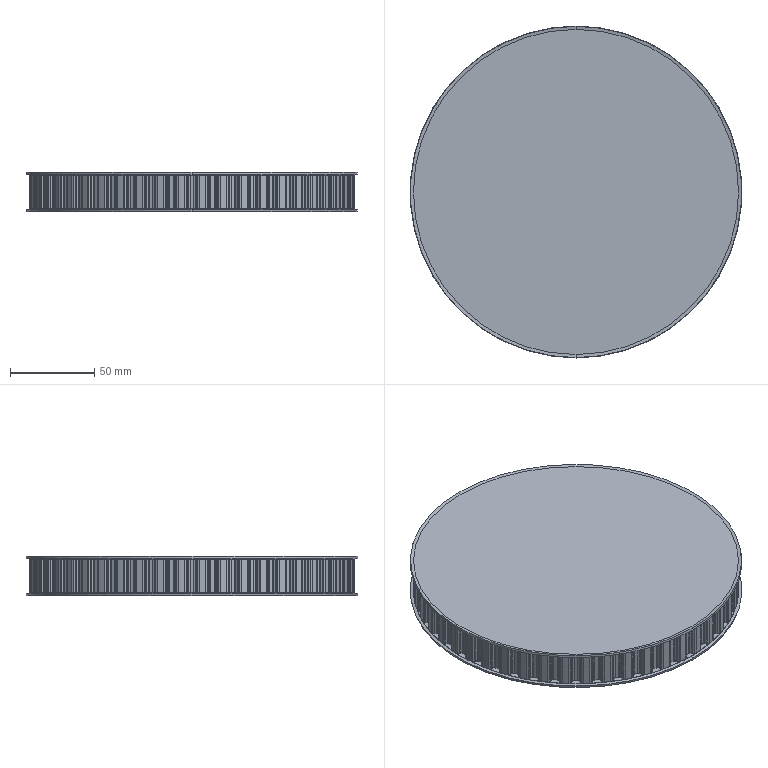Part | SolidWorks | features BaseBody 1 | 1 solid | 690 faces | box 196.734 x 196.734 x 23.179 mm | volume 644738 mm3 | cylinder 432 | plane 242 | cone 12 | torus 4 | commonest cylinder face diameters 3.2 x384 192.67 x48